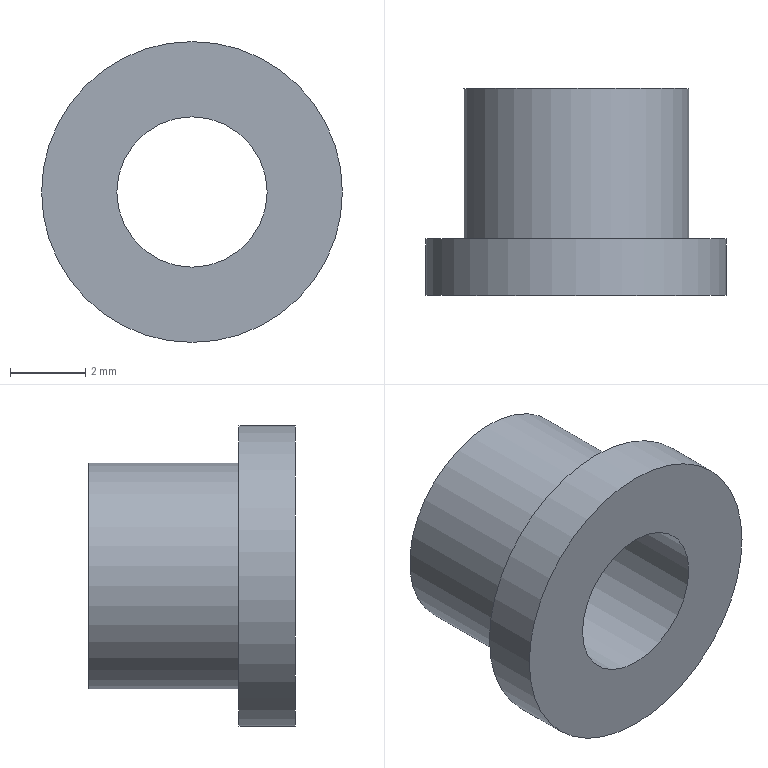Part | STEP file | 1-06.6 | 1 solid | 6 faces | box 8 x 5.5 x 8 mm | volume 119.381 mm3 | cylinder 3 | plane 3 | commonest cylinder face diameters 4 x1 6 x1 8 x1
STEP:
#1=CARTESIAN_POINT('',(0.,0.,0.));
#2=DIRECTION('',(0.,0.,1.));
#3=DIRECTION('',(1.,0.,0.));
#4=AXIS2_PLACEMENT_3D('',#1,#2,#3);
#5=CARTESIAN_POINT('',(4.,0.,0.));
#6=VERTEX_POINT('',#5);
#7=CARTESIAN_POINT('',(0.,0.,0.));
#8=DIRECTION('',(0.,-1.,0.));
#9=DIRECTION('',(1.,0.,0.));
#10=AXIS2_PLACEMENT_3D('',#7,#8,#9);
#11=CIRCLE('',#10,4.);
#12=CARTESIAN_POINT('',(0.,0.,0.));
#13=DIRECTION('',(0.,-1.,0.));
#14=DIRECTION('',(1.,0.,0.));
#15=AXIS2_PLACEMENT_3D('',#12,#13,#14);
#16=CYLINDRICAL_SURFACE('',#15,4.);
#17=CARTESIAN_POINT('',(0.,0.));
#18=DIRECTION('',(1.,0.));
#19=VECTOR('',#18,1.);
#20=LINE('',#17,#19);
#21=(GEOMETRIC_REPRESENTATION_CONTEXT(2)PARAMETRIC_REPRESENTATION_CONTEXT()REPRESENTATION_CONTEXT('',''));
#22=DEFINITIONAL_REPRESENTATION('',(#20),#21);
#23=PCURVE('',#16,#22);
#24=CARTESIAN_POINT('',(-1.072,0.,0.));
#25=DIRECTION('',(0.,-1.,0.));
#26=DIRECTION('',(1.,0.,0.));
#27=AXIS2_PLACEMENT_3D('',#24,#25,#26);
#28=PLANE('',#27);
#29=CARTESIAN_POINT('',(1.072,0.));
#30=DIRECTION('',(1.,0.));
#31=AXIS2_PLACEMENT_2D('',#29,#30);
#32=CIRCLE('',#31,4.);
#33=(GEOMETRIC_REPRESENTATION_CONTEXT(2)PARAMETRIC_REPRESENTATION_CONTEXT()REPRESENTATION_CONTEXT('',''));
#34=DEFINITIONAL_REPRESENTATION('',(#32),#33);
#35=PCURVE('',#28,#34);
#36=SURFACE_CURVE('',#11,(#23,#35),.PCURVE_S1.);
#37=EDGE_CURVE('',#6,#6,#36,.T.);
#38=ORIENTED_EDGE('',*,*,#37,.T.);
#39=CARTESIAN_POINT('',(4.,-1.5,0.));
#40=VERTEX_POINT('',#39);
#41=CARTESIAN_POINT('',(4.,0.,0.));
#42=DIRECTION('',(0.,-1.,0.));
#43=VECTOR('',#42,1.);
#44=LINE('',#41,#43);
#45=CARTESIAN_POINT('',(6.283,0.));
#46=DIRECTION('',(0.,1.));
#47=VECTOR('',#46,1.);
#48=LINE('',#45,#47);
#49=(GEOMETRIC_REPRESENTATION_CONTEXT(2)PARAMETRIC_REPRESENTATION_CONTEXT()REPRESENTATION_CONTEXT('',''));
#50=DEFINITIONAL_REPRESENTATION('',(#48),#49);
#51=PCURVE('',#16,#50);
#52=CARTESIAN_POINT('',(0.,0.));
#53=DIRECTION('',(0.,1.));
#54=VECTOR('',#53,1.);
#55=LINE('',#52,#54);
#56=(GEOMETRIC_REPRESENTATION_CONTEXT(2)PARAMETRIC_REPRESENTATION_CONTEXT()REPRESENTATION_CONTEXT('',''));
#57=DEFINITIONAL_REPRESENTATION('',(#55),#56);
#58=PCURVE('',#16,#57);
#59=SEAM_CURVE('',#44,(#51,#58),.PCURVE_S1.);
#60=EDGE_CURVE('',#6,#40,#59,.T.);
#61=ORIENTED_EDGE('',*,*,#60,.T.);
#62=CARTESIAN_POINT('',(0.,-1.5,0.));
#63=DIRECTION('',(0.,-1.,0.));
#64=DIRECTION('',(1.,0.,0.));
#65=AXIS2_PLACEMENT_3D('',#62,#63,#64);
#66=CIRCLE('',#65,4.);
#67=CARTESIAN_POINT('',(0.,1.5));
#68=DIRECTION('',(1.,0.));
#69=VECTOR('',#68,1.);
#70=LINE('',#67,#69);
#71=(GEOMETRIC_REPRESENTATION_CONTEXT(2)PARAMETRIC_REPRESENTATION_CONTEXT()REPRESENTATION_CONTEXT('',''));
#72=DEFINITIONAL_REPRESENTATION('',(#70),#71);
#73=PCURVE('',#16,#72);
#74=CARTESIAN_POINT('',(-1.072,-1.5,0.));
#75=DIRECTION('',(0.,-1.,0.));
#76=DIRECTION('',(1.,0.,0.));
#77=AXIS2_PLACEMENT_3D('',#74,#75,#76);
#78=PLANE('',#77);
#79=CARTESIAN_POINT('',(1.072,0.));
#80=DIRECTION('',(1.,0.));
#81=AXIS2_PLACEMENT_2D('',#79,#80);
#82=CIRCLE('',#81,4.);
#83=(GEOMETRIC_REPRESENTATION_CONTEXT(2)PARAMETRIC_REPRESENTATION_CONTEXT()REPRESENTATION_CONTEXT('',''));
#84=DEFINITIONAL_REPRESENTATION('',(#82),#83);
#85=PCURVE('',#78,#84);
#86=SURFACE_CURVE('',#66,(#73,#85),.PCURVE_S1.);
#87=EDGE_CURVE('',#40,#40,#86,.T.);
#88=ORIENTED_EDGE('',*,*,#87,.F.);
#89=ORIENTED_EDGE('',*,*,#60,.F.);
#90=EDGE_LOOP('',(#38,#61,#88,#89));
#91=FACE_BOUND('',#90,.T.);
#92=ADVANCED_FACE('',(#91),#16,.T.);
#93=ORIENTED_EDGE('',*,*,#37,.T.);
#94=EDGE_LOOP('',(#93));
#95=FACE_BOUND('',#94,.F.);
#96=CARTESIAN_POINT('',(3.,0.,0.));
#97=VERTEX_POINT('',#96);
#98=CARTESIAN_POINT('',(0.,0.,0.));
#99=DIRECTION('',(0.,-1.,0.));
#100=DIRECTION('',(1.,0.,0.));
#101=AXIS2_PLACEMENT_3D('',#98,#99,#100);
#102=CIRCLE('',#101,3.);
#103=CARTESIAN_POINT('',(1.072,0.));
#104=DIRECTION('',(1.,0.));
#105=AXIS2_PLACEMENT_2D('',#103,#104);
#106=CIRCLE('',#105,3.);
#107=(GEOMETRIC_REPRESENTATION_CONTEXT(2)PARAMETRIC_REPRESENTATION_CONTEXT()REPRESENTATION_CONTEXT('',''));
#108=DEFINITIONAL_REPRESENTATION('',(#106),#107);
#109=PCURVE('',#28,#108);
#110=CARTESIAN_POINT('',(0.,0.,0.));
#111=DIRECTION('',(0.,1.,0.));
#112=DIRECTION('',(1.,0.,0.));
#113=AXIS2_PLACEMENT_3D('',#110,#111,#112);
#114=CYLINDRICAL_SURFACE('',#113,3.);
#115=CARTESIAN_POINT('',(6.283,0.));
#116=DIRECTION('',(-1.,0.));
#117=VECTOR('',#116,1.);
#118=LINE('',#115,#117);
#119=(GEOMETRIC_REPRESENTATION_CONTEXT(2)PARAMETRIC_REPRESENTATION_CONTEXT()REPRESENTATION_CONTEXT('',''));
#120=DEFINITIONAL_REPRESENTATION('',(#118),#119);
#121=PCURVE('',#114,#120);
#122=SURFACE_CURVE('',#102,(#109,#121),.PCURVE_S1.);
#123=EDGE_CURVE('',#97,#97,#122,.T.);
#124=ORIENTED_EDGE('',*,*,#123,.F.);
#125=EDGE_LOOP('',(#124));
#126=FACE_BOUND('',#125,.F.);
#127=ADVANCED_FACE('',(#95,#126),#28,.F.);
#128=CARTESIAN_POINT('',(3.,4.,0.));
#129=VERTEX_POINT('',#128);
#130=CARTESIAN_POINT('',(3.,0.,0.));
#131=DIRECTION('',(0.,1.,0.));
#132=VECTOR('',#131,1.);
#133=LINE('',#130,#132);
#134=CARTESIAN_POINT('',(6.283,0.));
#135=DIRECTION('',(0.,1.));
#136=VECTOR('',#135,1.);
#137=LINE('',#134,#136);
#138=(GEOMETRIC_REPRESENTATION_CONTEXT(2)PARAMETRIC_REPRESENTATION_CONTEXT()REPRESENTATION_CONTEXT('',''));
#139=DEFINITIONAL_REPRESENTATION('',(#137),#138);
#140=PCURVE('',#114,#139);
#141=CARTESIAN_POINT('',(0.,0.));
#142=DIRECTION('',(0.,1.));
#143=VECTOR('',#142,1.);
#144=LINE('',#141,#143);
#145=(GEOMETRIC_REPRESENTATION_CONTEXT(2)PARAMETRIC_REPRESENTATION_CONTEXT()REPRESENTATION_CONTEXT('',''));
#146=DEFINITIONAL_REPRESENTATION('',(#144),#145);
#147=PCURVE('',#114,#146);
#148=SEAM_CURVE('',#133,(#140,#147),.PCURVE_S1.);
#149=EDGE_CURVE('',#97,#129,#148,.T.);
#150=ORIENTED_EDGE('',*,*,#149,.T.);
#151=CARTESIAN_POINT('',(0.,4.,0.));
#152=DIRECTION('',(0.,-1.,0.));
#153=DIRECTION('',(1.,0.,0.));
#154=AXIS2_PLACEMENT_3D('',#151,#152,#153);
#155=CIRCLE('',#154,3.);
#156=CARTESIAN_POINT('',(6.283,4.));
#157=DIRECTION('',(-1.,0.));
#158=VECTOR('',#157,1.);
#159=LINE('',#156,#158);
#160=(GEOMETRIC_REPRESENTATION_CONTEXT(2)PARAMETRIC_REPRESENTATION_CONTEXT()REPRESENTATION_CONTEXT('',''));
#161=DEFINITIONAL_REPRESENTATION('',(#159),#160);
#162=PCURVE('',#114,#161);
#163=CARTESIAN_POINT('',(-0.8038,4.,0.));
#164=DIRECTION('',(0.,-1.,0.));
#165=DIRECTION('',(1.,0.,0.));
#166=AXIS2_PLACEMENT_3D('',#163,#164,#165);
#167=PLANE('',#166);
#168=CARTESIAN_POINT('',(0.8038,0.));
#169=DIRECTION('',(1.,0.));
#170=AXIS2_PLACEMENT_2D('',#168,#169);
#171=CIRCLE('',#170,3.);
#172=(GEOMETRIC_REPRESENTATION_CONTEXT(2)PARAMETRIC_REPRESENTATION_CONTEXT()REPRESENTATION_CONTEXT('',''));
#173=DEFINITIONAL_REPRESENTATION('',(#171),#172);
#174=PCURVE('',#167,#173);
#175=SURFACE_CURVE('',#155,(#162,#174),.PCURVE_S1.);
#176=EDGE_CURVE('',#129,#129,#175,.T.);
#177=ORIENTED_EDGE('',*,*,#176,.T.);
#178=ORIENTED_EDGE('',*,*,#149,.F.);
#179=ORIENTED_EDGE('',*,*,#123,.F.);
#180=EDGE_LOOP('',(#150,#177,#178,#179));
#181=FACE_BOUND('',#180,.T.);
#182=ADVANCED_FACE('',(#181),#114,.T.);
#183=ORIENTED_EDGE('',*,*,#87,.T.);
#184=EDGE_LOOP('',(#183));
#185=FACE_BOUND('',#184,.T.);
#186=CARTESIAN_POINT('',(2.,-1.5,0.));
#187=VERTEX_POINT('',#186);
#188=CARTESIAN_POINT('',(0.,-1.5,0.));
#189=DIRECTION('',(0.,-1.,0.));
#190=DIRECTION('',(1.,0.,0.));
#191=AXIS2_PLACEMENT_3D('',#188,#189,#190);
#192=CIRCLE('',#191,2.);
#193=CARTESIAN_POINT('',(1.072,0.));
#194=DIRECTION('',(1.,0.));
#195=AXIS2_PLACEMENT_2D('',#193,#194);
#196=CIRCLE('',#195,2.);
#197=(GEOMETRIC_REPRESENTATION_CONTEXT(2)PARAMETRIC_REPRESENTATION_CONTEXT()REPRESENTATION_CONTEXT('',''));
#198=DEFINITIONAL_REPRESENTATION('',(#196),#197);
#199=PCURVE('',#78,#198);
#200=CARTESIAN_POINT('',(0.,-1.5,0.));
#201=DIRECTION('',(0.,1.,0.));
#202=DIRECTION('',(1.,0.,0.));
#203=AXIS2_PLACEMENT_3D('',#200,#201,#202);
#204=CYLINDRICAL_SURFACE('',#203,2.);
#205=CARTESIAN_POINT('',(6.283,0.));
#206=DIRECTION('',(-1.,0.));
#207=VECTOR('',#206,1.);
#208=LINE('',#205,#207);
#209=(GEOMETRIC_REPRESENTATION_CONTEXT(2)PARAMETRIC_REPRESENTATION_CONTEXT()REPRESENTATION_CONTEXT('',''));
#210=DEFINITIONAL_REPRESENTATION('',(#208),#209);
#211=PCURVE('',#204,#210);
#212=SURFACE_CURVE('',#192,(#199,#211),.PCURVE_S1.);
#213=EDGE_CURVE('',#187,#187,#212,.T.);
#214=ORIENTED_EDGE('',*,*,#213,.F.);
#215=EDGE_LOOP('',(#214));
#216=FACE_BOUND('',#215,.T.);
#217=ADVANCED_FACE('',(#185,#216),#78,.T.);
#218=ORIENTED_EDGE('',*,*,#176,.T.);
#219=EDGE_LOOP('',(#218));
#220=FACE_BOUND('',#219,.F.);
#221=CARTESIAN_POINT('',(2.,4.,0.));
#222=VERTEX_POINT('',#221);
#223=CARTESIAN_POINT('',(0.,4.,0.));
#224=DIRECTION('',(0.,1.,0.));
#225=DIRECTION('',(1.,0.,0.));
#226=AXIS2_PLACEMENT_3D('',#223,#224,#225);
#227=CIRCLE('',#226,2.);
#228=CARTESIAN_POINT('',(2.804,0.));
#229=CARTESIAN_POINT('',(2.804,-3.464));
#230=CARTESIAN_POINT('',(-0.1962,-1.732));
#231=CARTESIAN_POINT('',(-3.196,0.));
#232=CARTESIAN_POINT('',(-0.1962,1.732));
#233=CARTESIAN_POINT('',(2.804,3.464));
#234=CARTESIAN_POINT('',(2.804,0.));
#235=(BOUNDED_CURVE()B_SPLINE_CURVE(2,(#228,#229,#230,#231,#232,#233,#234),.UNSPECIFIED.,.T.,.F.)B_SPLINE_CURVE_WITH_KNOTS((1,2,2,2,2,1),(-2.094,0.,2.094,4.189,6.283,8.378),.UNSPECIFIED.)CURVE()GEOMETRIC_REPRESENTATION_ITEM()RATIONAL_B_SPLINE_CURVE((1.,0.5,1.,0.5,1.,0.5,1.))REPRESENTATION_ITEM(''));
#236=(GEOMETRIC_REPRESENTATION_CONTEXT(2)PARAMETRIC_REPRESENTATION_CONTEXT()REPRESENTATION_CONTEXT('',''));
#237=DEFINITIONAL_REPRESENTATION('',(#235),#236);
#238=PCURVE('',#167,#237);
#239=CARTESIAN_POINT('',(0.,5.5));
#240=DIRECTION('',(1.,0.));
#241=VECTOR('',#240,1.);
#242=LINE('',#239,#241);
#243=(GEOMETRIC_REPRESENTATION_CONTEXT(2)PARAMETRIC_REPRESENTATION_CONTEXT()REPRESENTATION_CONTEXT('',''));
#244=DEFINITIONAL_REPRESENTATION('',(#242),#243);
#245=PCURVE('',#204,#244);
#246=SURFACE_CURVE('',#227,(#238,#245),.PCURVE_S1.);
#247=EDGE_CURVE('',#222,#222,#246,.T.);
#248=ORIENTED_EDGE('',*,*,#247,.T.);
#249=EDGE_LOOP('',(#248));
#250=FACE_BOUND('',#249,.F.);
#251=ADVANCED_FACE('',(#220,#250),#167,.F.);
#252=CARTESIAN_POINT('',(2.,-1.5,0.));
#253=DIRECTION('',(0.,1.,0.));
#254=VECTOR('',#253,1.);
#255=LINE('',#252,#254);
#256=CARTESIAN_POINT('',(6.283,0.));
#257=DIRECTION('',(0.,1.));
#258=VECTOR('',#257,1.);
#259=LINE('',#256,#258);
#260=(GEOMETRIC_REPRESENTATION_CONTEXT(2)PARAMETRIC_REPRESENTATION_CONTEXT()REPRESENTATION_CONTEXT('',''));
#261=DEFINITIONAL_REPRESENTATION('',(#259),#260);
#262=PCURVE('',#204,#261);
#263=CARTESIAN_POINT('',(0.,0.));
#264=DIRECTION('',(0.,1.));
#265=VECTOR('',#264,1.);
#266=LINE('',#263,#265);
#267=(GEOMETRIC_REPRESENTATION_CONTEXT(2)PARAMETRIC_REPRESENTATION_CONTEXT()REPRESENTATION_CONTEXT('',''));
#268=DEFINITIONAL_REPRESENTATION('',(#266),#267);
#269=PCURVE('',#204,#268);
#270=SEAM_CURVE('',#255,(#262,#269),.PCURVE_S1.);
#271=EDGE_CURVE('',#187,#222,#270,.T.);
#272=ORIENTED_EDGE('',*,*,#271,.T.);
#273=ORIENTED_EDGE('',*,*,#247,.F.);
#274=ORIENTED_EDGE('',*,*,#271,.F.);
#275=ORIENTED_EDGE('',*,*,#213,.F.);
#276=EDGE_LOOP('',(#272,#273,#274,#275));
#277=FACE_BOUND('',#276,.F.);
#278=ADVANCED_FACE('',(#277),#204,.F.);
#279=CLOSED_SHELL('',(#92,#127,#182,#217,#251,#278));
#280=MANIFOLD_SOLID_BREP('',#279);
#281=(LENGTH_UNIT()NAMED_UNIT(*)SI_UNIT(.MILLI.,.METRE.));
#282=UNCERTAINTY_MEASURE_WITH_UNIT(LENGTH_MEASURE(0.0000001),#281,'','');
#283=(NAMED_UNIT(*)PLANE_ANGLE_UNIT()SI_UNIT($,.RADIAN.));
#284=(NAMED_UNIT(*)SI_UNIT($,.STERADIAN.)SOLID_ANGLE_UNIT());
#285=(GEOMETRIC_REPRESENTATION_CONTEXT(3)GLOBAL_UNCERTAINTY_ASSIGNED_CONTEXT((#282))GLOBAL_UNIT_ASSIGNED_CONTEXT((#281,#283,#284))REPRESENTATION_CONTEXT('',''));
#286=ADVANCED_BREP_SHAPE_REPRESENTATION('',(#4,#280),#285);